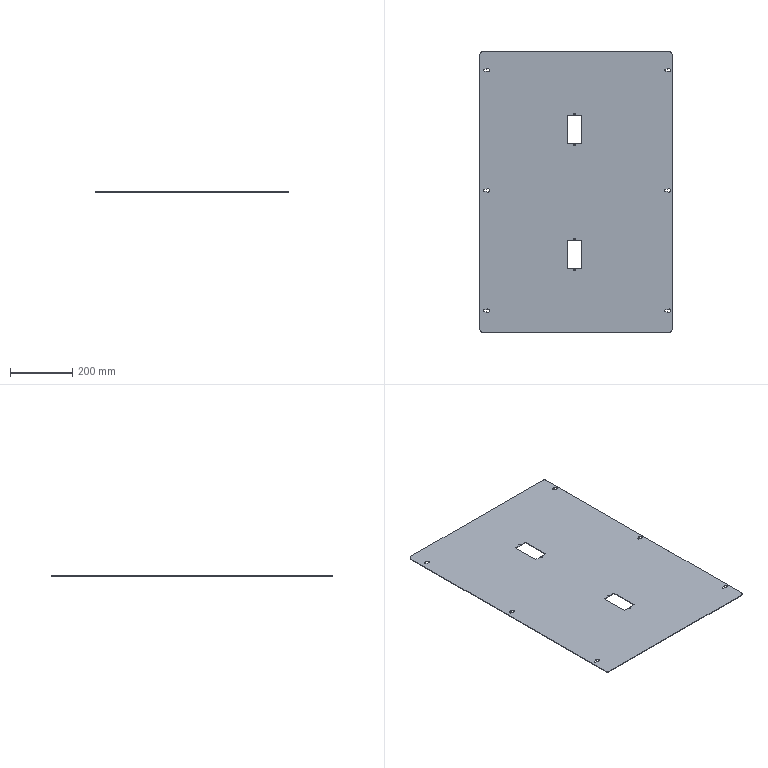Part | SolidWorks | features ICE 4, Extrusion 1, Fillet 1, HoleWzd 1, LPattern 1 | 1 solid | 56 faces | box 615 x 900 x 2 mm | volume 1088591 mm3 | cylinder 30 | plane 26 | commonest cylinder face diameters 6.6 x12 4.5 x8 11 x6 20 x4